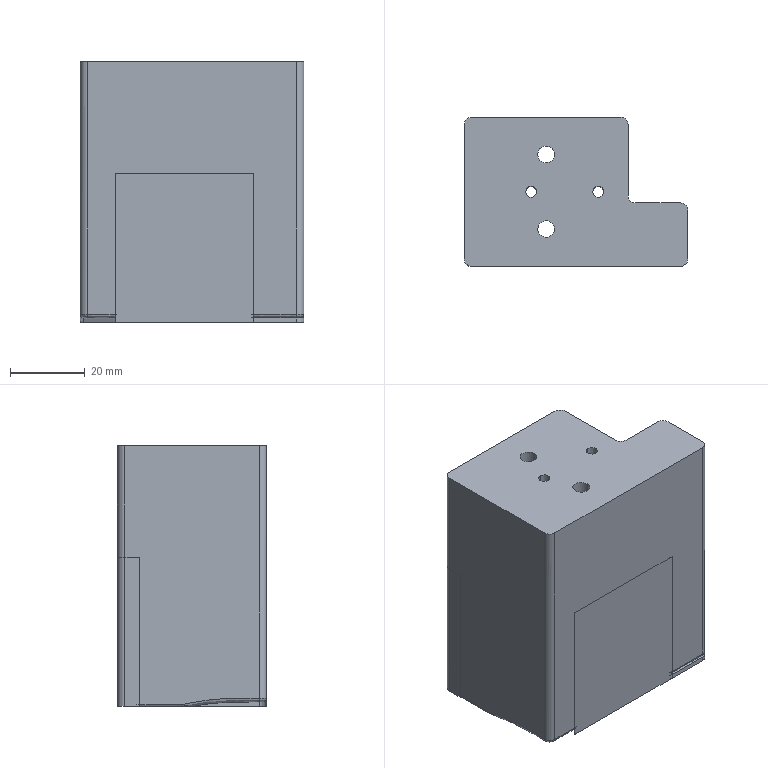NC program | NX | posted with a generic post | part box 60.004 x 40.015 x 70 mm
Whole program:
N10 G17 G21 G94 G90
(DRILLING_COPY , TOOL : D4A45)
N12 T02 M6
N14 G54
N16 G17 G0 G90 X-8. Y10. B0. C0. S5000 M3
N18 G43 Z30. H2
N20 G94 G81 G98 Z-1. F250. R3.
N22 Y-10.
N24 X6. Y0.
N26 X-12.
N28 G80
N30 G0 X-12. Y0. Z30.
N32 M5
(DRILLING_COPY_COPY_COPY_COPY_COPY , TOOL : 3.0ZT)
N34 T13 M6
N36 G54
N38 G17 G0 G90 X6. Y0. B0. C0. S1910 M3
N40 G43 Z30. H13
N42 G94 G83 G98 Z-32.401 F180. Q2. R3.
N44 X-12.
N46 G80
N48 G0 X-12. Y0. Z30.
N50 M5
(DRILLING_COPY_COPY_COPY_COPY_COPY_COPY , TOOL : 4.5ZT)
N52 T15 M6
N54 G54
N56 G17 G0 G90 X-8. Y10. B0. C0. S1910 M3
N58 G43 Z30. H15
N60 G94 G83 G98 Z-32.352 F180. Q2. R3.
N62 Y-10.
N64 G80
N66 G0 X-8. Y-10. Z30.
N68 M5
(ZLEVEL_PROFILE_1_COPY_1_COPY_COPY , TOOL : D4A45)
N70 T02 M6
N72 G54
N74 G17 G0 G90 X-12. Y0.541 B0. C0. S9500 M3
N76 G43 Z30. H2
N78 Z1.
N80 G94 G1 Z-1. F1000.
N82 X-12.002
N84 G3 X-12.541 Y-0.002 R0.541
N86 X-12. Y0.541 R-0.541
N88 X-12.346 Y0.341 R0.4
N90 G1 Z0.
N92 G0 Z30.
N94 X-7.851 Y10.468
N96 Z0.
N98 G1 Z-1.
N100 X-7.654 Y11.091
N102 G3 X-8. Y11.291 R0.4
N104 X-9.291 Y10. R1.291
N106 X-8. Y11.291 R-1.291
N108 X-8.346 Y11.091 R0.4
N110 G1 X-8.149 Y10.468
N112 Z0.
N114 G0 Z30.
N116 Y-10.468
N118 Z0.
N120 G1 Z-1.
N122 X-8.346 Y-11.091
N124 G3 X-8. Y-11.291 R0.4
N126 X-6.709 Y-10. R1.291
N128 X-8. Y-11.291 R-1.291
N130 X-7.654 Y-11.091 R0.4
N132 G1 X-7.851 Y-10.468
N134 Z0.
N136 G0 Z30.
N138 X6. Y0.541
N140 Z1.
N142 G1 Z-1.
N144 X5.999
N146 G3 X5.459 Y-0.001 R0.541
N148 X6. Y0.541 R-0.541
N150 X5.654 Y0.341 R0.4
N152 G1 Z0.
N154 G0 Z30.
N156 X28.659 Y-21.7
N158 Z0.
N160 G1 Z-1.
N162 X28.346 Y-21.159
N164 G3 X28. Y-20.959 R0.4
N166 G1 X-28.
N168 G2 X-30.959 Y-18. R2.959
N170 G1 Y18.
N172 G2 X-28. Y20.959 R2.959
N174 G1 X12.
N176 G2 X14.959 Y18. R2.959
N178 G1 Y-1.
N180 G3 X16. Y-2.041 R1.041
N182 G1 X28.
N184 G2 X30.959 Y-5. R2.959
N186 G1 Y-18.
N188 G2 X28. Y-20.959 R2.959
N190 G3 X27.654 Y-21.159 R0.4
N192 G1 X27.307 Y-21.759
N194 Z0.
N196 G0 Z30.
N198 M5
N200 M2